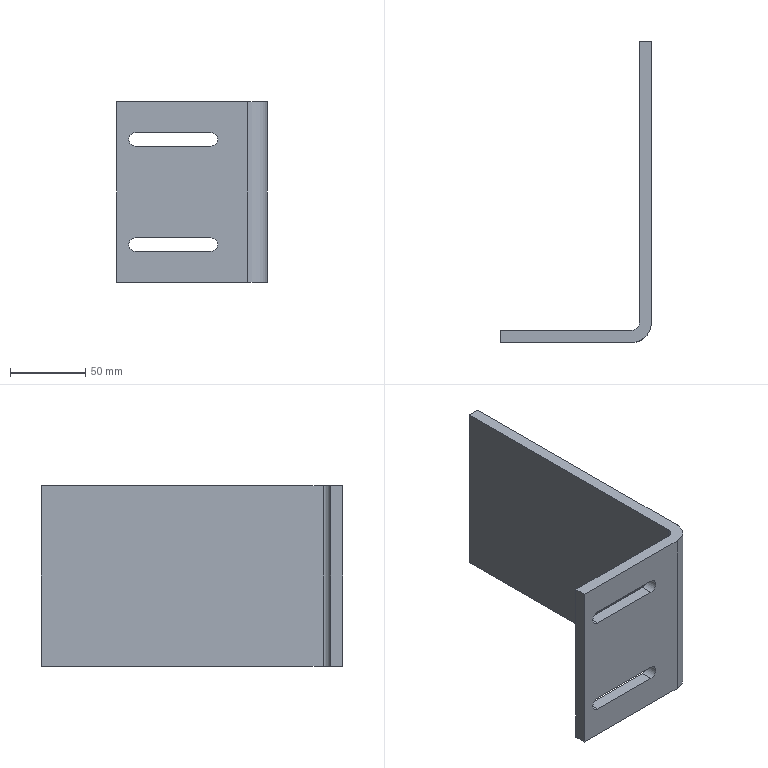Part | SolidWorks | features Extrusion 1, ICE 1 | 1 solid | 18 faces | box 100 x 200 x 120 mm | volume 268394 mm3 | plane 12 | cylinder 6 | commonest cylinder face diameters 9 x4 10 x1 26 x1
STEP:
#1=CARTESIAN_POINT('',(12.5,8.,20.5));
#2=VERTEX_POINT('',#1);
#3=CARTESIAN_POINT('',(12.5,8.,29.5));
#4=VERTEX_POINT('',#3);
#5=CARTESIAN_POINT('',(12.5,8.,25.));
#6=DIRECTION('',(0.,1.,0.));
#7=DIRECTION('',(0.,0.,1.));
#8=AXIS2_PLACEMENT_3D('',#5,#6,#7);
#9=CIRCLE('',#8,4.5);
#10=EDGE_CURVE('',#2,#4,#9,.T.);
#11=ORIENTED_EDGE('',*,*,#10,.F.);
#12=CARTESIAN_POINT('',(62.5,8.,20.5));
#13=VERTEX_POINT('',#12);
#14=CARTESIAN_POINT('',(12.5,8.,20.5));
#15=DIRECTION('',(-1.,0.,0.));
#16=VECTOR('',#15,1000.);
#17=LINE('',#14,#16);
#18=EDGE_CURVE('',#13,#2,#17,.T.);
#19=ORIENTED_EDGE('',*,*,#18,.F.);
#20=CARTESIAN_POINT('',(62.5,8.,29.5));
#21=VERTEX_POINT('',#20);
#22=CARTESIAN_POINT('',(62.5,8.,25.));
#23=DIRECTION('',(0.,1.,0.));
#24=DIRECTION('',(0.,0.,1.));
#25=AXIS2_PLACEMENT_3D('',#22,#23,#24);
#26=CIRCLE('',#25,4.5);
#27=EDGE_CURVE('',#21,#13,#26,.T.);
#28=ORIENTED_EDGE('',*,*,#27,.F.);
#29=CARTESIAN_POINT('',(12.5,8.,29.5));
#30=DIRECTION('',(1.,0.,0.));
#31=VECTOR('',#30,1000.);
#32=LINE('',#29,#31);
#33=EDGE_CURVE('',#4,#21,#32,.T.);
#34=ORIENTED_EDGE('',*,*,#33,.F.);
#35=EDGE_LOOP('',(#11,#19,#28,#34));
#36=FACE_BOUND('',#35,.T.);
#37=CARTESIAN_POINT('',(12.5,8.,90.5));
#38=VERTEX_POINT('',#37);
#39=CARTESIAN_POINT('',(12.5,8.,99.5));
#40=VERTEX_POINT('',#39);
#41=CARTESIAN_POINT('',(12.5,8.,95.));
#42=DIRECTION('',(0.,1.,0.));
#43=DIRECTION('',(0.,0.,-1.));
#44=AXIS2_PLACEMENT_3D('',#41,#42,#43);
#45=CIRCLE('',#44,4.5);
#46=EDGE_CURVE('',#38,#40,#45,.T.);
#47=ORIENTED_EDGE('',*,*,#46,.F.);
#48=CARTESIAN_POINT('',(62.5,8.,90.5));
#49=VERTEX_POINT('',#48);
#50=CARTESIAN_POINT('',(12.5,8.,90.5));
#51=DIRECTION('',(-1.,0.,0.));
#52=VECTOR('',#51,1000.);
#53=LINE('',#50,#52);
#54=EDGE_CURVE('',#49,#38,#53,.T.);
#55=ORIENTED_EDGE('',*,*,#54,.F.);
#56=CARTESIAN_POINT('',(62.5,8.,99.5));
#57=VERTEX_POINT('',#56);
#58=CARTESIAN_POINT('',(62.5,8.,95.));
#59=DIRECTION('',(0.,1.,0.));
#60=DIRECTION('',(0.,0.,-1.));
#61=AXIS2_PLACEMENT_3D('',#58,#59,#60);
#62=CIRCLE('',#61,4.5);
#63=EDGE_CURVE('',#57,#49,#62,.T.);
#64=ORIENTED_EDGE('',*,*,#63,.F.);
#65=CARTESIAN_POINT('',(12.5,8.,99.5));
#66=DIRECTION('',(1.,0.,0.));
#67=VECTOR('',#66,1000.);
#68=LINE('',#65,#67);
#69=EDGE_CURVE('',#40,#57,#68,.T.);
#70=ORIENTED_EDGE('',*,*,#69,.F.);
#71=EDGE_LOOP('',(#47,#55,#64,#70));
#72=FACE_BOUND('',#71,.T.);
#73=CARTESIAN_POINT('',(0.,8.,0.));
#74=VERTEX_POINT('',#73);
#75=CARTESIAN_POINT('',(87.,8.,0.));
#76=VERTEX_POINT('',#75);
#77=CARTESIAN_POINT('',(0.,8.,0.));
#78=DIRECTION('',(1.,0.,0.));
#79=VECTOR('',#78,1000.);
#80=LINE('',#77,#79);
#81=EDGE_CURVE('',#74,#76,#80,.T.);
#82=ORIENTED_EDGE('',*,*,#81,.F.);
#83=CARTESIAN_POINT('',(0.,8.,120.));
#84=VERTEX_POINT('',#83);
#85=CARTESIAN_POINT('',(0.,8.,120.));
#86=DIRECTION('',(0.,0.,-1.));
#87=VECTOR('',#86,1000.);
#88=LINE('',#85,#87);
#89=EDGE_CURVE('',#84,#74,#88,.T.);
#90=ORIENTED_EDGE('',*,*,#89,.F.);
#91=CARTESIAN_POINT('',(87.,8.,120.));
#92=VERTEX_POINT('',#91);
#93=CARTESIAN_POINT('',(0.,8.,120.));
#94=DIRECTION('',(1.,0.,0.));
#95=VECTOR('',#94,1000.);
#96=LINE('',#93,#95);
#97=EDGE_CURVE('',#84,#92,#96,.T.);
#98=ORIENTED_EDGE('',*,*,#97,.T.);
#99=CARTESIAN_POINT('',(87.,8.,120.));
#100=DIRECTION('',(0.,0.,-1.));
#101=VECTOR('',#100,1000.);
#102=LINE('',#99,#101);
#103=EDGE_CURVE('',#92,#76,#102,.T.);
#104=ORIENTED_EDGE('',*,*,#103,.T.);
#105=EDGE_LOOP('',(#82,#90,#98,#104));
#106=FACE_OUTER_BOUND('',#105,.T.);
#107=CARTESIAN_POINT('',(0.,8.,120.));
#108=DIRECTION('',(0.,1.,0.));
#109=DIRECTION('',(0.,0.,1.));
#110=AXIS2_PLACEMENT_3D('',#107,#108,#109);
#111=PLANE('',#110);
#112=ADVANCED_FACE('',(#36,#72,#106),#111,.T.);
#113=CARTESIAN_POINT('',(0.,0.,0.));
#114=VERTEX_POINT('',#113);
#115=CARTESIAN_POINT('',(0.,8.,0.));
#116=DIRECTION('',(0.,-1.,0.));
#117=VECTOR('',#116,1000.);
#118=LINE('',#115,#117);
#119=EDGE_CURVE('',#74,#114,#118,.T.);
#120=ORIENTED_EDGE('',*,*,#119,.T.);
#121=CARTESIAN_POINT('',(0.,0.,120.));
#122=VERTEX_POINT('',#121);
#123=CARTESIAN_POINT('',(0.,0.,120.));
#124=DIRECTION('',(0.,0.,-1.));
#125=VECTOR('',#124,1000.);
#126=LINE('',#123,#125);
#127=EDGE_CURVE('',#122,#114,#126,.T.);
#128=ORIENTED_EDGE('',*,*,#127,.F.);
#129=CARTESIAN_POINT('',(0.,8.,120.));
#130=DIRECTION('',(0.,-1.,0.));
#131=VECTOR('',#130,1000.);
#132=LINE('',#129,#131);
#133=EDGE_CURVE('',#84,#122,#132,.T.);
#134=ORIENTED_EDGE('',*,*,#133,.F.);
#135=ORIENTED_EDGE('',*,*,#89,.T.);
#136=EDGE_LOOP('',(#120,#128,#134,#135));
#137=FACE_OUTER_BOUND('',#136,.T.);
#138=CARTESIAN_POINT('',(0.,8.,120.));
#139=DIRECTION('',(1.,0.,0.));
#140=DIRECTION('',(0.,0.,-1.));
#141=AXIS2_PLACEMENT_3D('',#138,#139,#140);
#142=PLANE('',#141);
#143=ADVANCED_FACE('',(#137),#142,.F.);
#144=CARTESIAN_POINT('',(62.5,0.,20.5));
#145=VERTEX_POINT('',#144);
#146=CARTESIAN_POINT('',(12.5,0.,20.5));
#147=VERTEX_POINT('',#146);
#148=CARTESIAN_POINT('',(0.,0.,20.5));
#149=DIRECTION('',(-1.,0.,0.));
#150=VECTOR('',#149,1000.);
#151=LINE('',#148,#150);
#152=EDGE_CURVE('',#145,#147,#151,.T.);
#153=ORIENTED_EDGE('',*,*,#152,.T.);
#154=CARTESIAN_POINT('',(12.5,0.,29.5));
#155=VERTEX_POINT('',#154);
#156=CARTESIAN_POINT('',(12.5,0.,25.));
#157=DIRECTION('',(0.,1.,0.));
#158=DIRECTION('',(0.,0.,1.));
#159=AXIS2_PLACEMENT_3D('',#156,#157,#158);
#160=CIRCLE('',#159,4.5);
#161=EDGE_CURVE('',#147,#155,#160,.T.);
#162=ORIENTED_EDGE('',*,*,#161,.T.);
#163=CARTESIAN_POINT('',(62.5,0.,29.5));
#164=VERTEX_POINT('',#163);
#165=CARTESIAN_POINT('',(0.,0.,29.5));
#166=DIRECTION('',(1.,0.,0.));
#167=VECTOR('',#166,1000.);
#168=LINE('',#165,#167);
#169=EDGE_CURVE('',#155,#164,#168,.T.);
#170=ORIENTED_EDGE('',*,*,#169,.T.);
#171=CARTESIAN_POINT('',(62.5,0.,25.));
#172=DIRECTION('',(0.,1.,0.));
#173=DIRECTION('',(0.,0.,1.));
#174=AXIS2_PLACEMENT_3D('',#171,#172,#173);
#175=CIRCLE('',#174,4.5);
#176=EDGE_CURVE('',#164,#145,#175,.T.);
#177=ORIENTED_EDGE('',*,*,#176,.T.);
#178=EDGE_LOOP('',(#153,#162,#170,#177));
#179=FACE_BOUND('',#178,.T.);
#180=CARTESIAN_POINT('',(62.5,0.,90.5));
#181=VERTEX_POINT('',#180);
#182=CARTESIAN_POINT('',(12.5,0.,90.5));
#183=VERTEX_POINT('',#182);
#184=CARTESIAN_POINT('',(0.,0.,90.5));
#185=DIRECTION('',(-1.,0.,0.));
#186=VECTOR('',#185,1000.);
#187=LINE('',#184,#186);
#188=EDGE_CURVE('',#181,#183,#187,.T.);
#189=ORIENTED_EDGE('',*,*,#188,.T.);
#190=CARTESIAN_POINT('',(12.5,0.,99.5));
#191=VERTEX_POINT('',#190);
#192=CARTESIAN_POINT('',(12.5,0.,95.));
#193=DIRECTION('',(0.,1.,0.));
#194=DIRECTION('',(0.,0.,1.));
#195=AXIS2_PLACEMENT_3D('',#192,#193,#194);
#196=CIRCLE('',#195,4.5);
#197=EDGE_CURVE('',#183,#191,#196,.T.);
#198=ORIENTED_EDGE('',*,*,#197,.T.);
#199=CARTESIAN_POINT('',(62.5,0.,99.5));
#200=VERTEX_POINT('',#199);
#201=CARTESIAN_POINT('',(0.,0.,99.5));
#202=DIRECTION('',(1.,0.,0.));
#203=VECTOR('',#202,1000.);
#204=LINE('',#201,#203);
#205=EDGE_CURVE('',#191,#200,#204,.T.);
#206=ORIENTED_EDGE('',*,*,#205,.T.);
#207=CARTESIAN_POINT('',(62.5,0.,95.));
#208=DIRECTION('',(0.,1.,0.));
#209=DIRECTION('',(0.,0.,1.));
#210=AXIS2_PLACEMENT_3D('',#207,#208,#209);
#211=CIRCLE('',#210,4.5);
#212=EDGE_CURVE('',#200,#181,#211,.T.);
#213=ORIENTED_EDGE('',*,*,#212,.T.);
#214=EDGE_LOOP('',(#189,#198,#206,#213));
#215=FACE_BOUND('',#214,.T.);
#216=CARTESIAN_POINT('',(87.,0.,0.));
#217=VERTEX_POINT('',#216);
#218=CARTESIAN_POINT('',(0.,0.,0.));
#219=DIRECTION('',(1.,0.,0.));
#220=VECTOR('',#219,1000.);
#221=LINE('',#218,#220);
#222=EDGE_CURVE('',#114,#217,#221,.T.);
#223=ORIENTED_EDGE('',*,*,#222,.T.);
#224=CARTESIAN_POINT('',(87.,0.,120.));
#225=VERTEX_POINT('',#224);
#226=CARTESIAN_POINT('',(87.,0.,120.));
#227=DIRECTION('',(0.,0.,-1.));
#228=VECTOR('',#227,1000.);
#229=LINE('',#226,#228);
#230=EDGE_CURVE('',#225,#217,#229,.T.);
#231=ORIENTED_EDGE('',*,*,#230,.F.);
#232=CARTESIAN_POINT('',(0.,0.,120.));
#233=DIRECTION('',(1.,0.,0.));
#234=VECTOR('',#233,1000.);
#235=LINE('',#232,#234);
#236=EDGE_CURVE('',#122,#225,#235,.T.);
#237=ORIENTED_EDGE('',*,*,#236,.F.);
#238=ORIENTED_EDGE('',*,*,#127,.T.);
#239=EDGE_LOOP('',(#223,#231,#237,#238));
#240=FACE_OUTER_BOUND('',#239,.T.);
#241=CARTESIAN_POINT('',(0.,0.,120.));
#242=DIRECTION('',(0.,1.,0.));
#243=DIRECTION('',(0.,0.,1.));
#244=AXIS2_PLACEMENT_3D('',#241,#242,#243);
#245=PLANE('',#244);
#246=ADVANCED_FACE('',(#179,#215,#240),#245,.F.);
#247=CARTESIAN_POINT('',(100.,13.,0.));
#248=VERTEX_POINT('',#247);
#249=CARTESIAN_POINT('',(87.,13.,0.));
#250=DIRECTION('',(0.,0.,1.));
#251=DIRECTION('',(1.,0.,0.));
#252=AXIS2_PLACEMENT_3D('',#249,#250,#251);
#253=CIRCLE('',#252,13.);
#254=EDGE_CURVE('',#217,#248,#253,.T.);
#255=ORIENTED_EDGE('',*,*,#254,.T.);
#256=CARTESIAN_POINT('',(100.,13.,120.));
#257=VERTEX_POINT('',#256);
#258=CARTESIAN_POINT('',(100.,13.,120.));
#259=DIRECTION('',(0.,0.,-1.));
#260=VECTOR('',#259,1000.);
#261=LINE('',#258,#260);
#262=EDGE_CURVE('',#257,#248,#261,.T.);
#263=ORIENTED_EDGE('',*,*,#262,.F.);
#264=CARTESIAN_POINT('',(87.,13.,120.));
#265=DIRECTION('',(0.,0.,1.));
#266=DIRECTION('',(1.,0.,0.));
#267=AXIS2_PLACEMENT_3D('',#264,#265,#266);
#268=CIRCLE('',#267,13.);
#269=EDGE_CURVE('',#225,#257,#268,.T.);
#270=ORIENTED_EDGE('',*,*,#269,.F.);
#271=ORIENTED_EDGE('',*,*,#230,.T.);
#272=EDGE_LOOP('',(#255,#263,#270,#271));
#273=FACE_OUTER_BOUND('',#272,.T.);
#274=CARTESIAN_POINT('',(87.,13.,120.));
#275=DIRECTION('',(0.,0.,-1.));
#276=DIRECTION('',(-1.,0.,0.));
#277=AXIS2_PLACEMENT_3D('',#274,#275,#276);
#278=CYLINDRICAL_SURFACE('',#277,13.);
#279=ADVANCED_FACE('',(#273),#278,.T.);
#280=CARTESIAN_POINT('',(100.,200.,0.));
#281=VERTEX_POINT('',#280);
#282=CARTESIAN_POINT('',(100.,13.,0.));
#283=DIRECTION('',(0.,1.,0.));
#284=VECTOR('',#283,1000.);
#285=LINE('',#282,#284);
#286=EDGE_CURVE('',#248,#281,#285,.T.);
#287=ORIENTED_EDGE('',*,*,#286,.T.);
#288=CARTESIAN_POINT('',(100.,200.,120.));
#289=VERTEX_POINT('',#288);
#290=CARTESIAN_POINT('',(100.,200.,120.));
#291=DIRECTION('',(0.,0.,-1.));
#292=VECTOR('',#291,1000.);
#293=LINE('',#290,#292);
#294=EDGE_CURVE('',#289,#281,#293,.T.);
#295=ORIENTED_EDGE('',*,*,#294,.F.);
#296=CARTESIAN_POINT('',(100.,13.,120.));
#297=DIRECTION('',(0.,1.,0.));
#298=VECTOR('',#297,1000.);
#299=LINE('',#296,#298);
#300=EDGE_CURVE('',#257,#289,#299,.T.);
#301=ORIENTED_EDGE('',*,*,#300,.F.);
#302=ORIENTED_EDGE('',*,*,#262,.T.);
#303=EDGE_LOOP('',(#287,#295,#301,#302));
#304=FACE_OUTER_BOUND('',#303,.T.);
#305=CARTESIAN_POINT('',(100.,13.,120.));
#306=DIRECTION('',(-1.,0.,0.));
#307=DIRECTION('',(0.,0.,1.));
#308=AXIS2_PLACEMENT_3D('',#305,#306,#307);
#309=PLANE('',#308);
#310=ADVANCED_FACE('',(#304),#309,.F.);
#311=CARTESIAN_POINT('',(92.,200.,0.));
#312=VERTEX_POINT('',#311);
#313=CARTESIAN_POINT('',(100.,200.,0.));
#314=DIRECTION('',(-1.,0.,0.));
#315=VECTOR('',#314,1000.);
#316=LINE('',#313,#315);
#317=EDGE_CURVE('',#281,#312,#316,.T.);
#318=ORIENTED_EDGE('',*,*,#317,.T.);
#319=CARTESIAN_POINT('',(92.,200.,120.));
#320=VERTEX_POINT('',#319);
#321=CARTESIAN_POINT('',(92.,200.,120.));
#322=DIRECTION('',(0.,0.,-1.));
#323=VECTOR('',#322,1000.);
#324=LINE('',#321,#323);
#325=EDGE_CURVE('',#320,#312,#324,.T.);
#326=ORIENTED_EDGE('',*,*,#325,.F.);
#327=CARTESIAN_POINT('',(100.,200.,120.));
#328=DIRECTION('',(-1.,0.,0.));
#329=VECTOR('',#328,1000.);
#330=LINE('',#327,#329);
#331=EDGE_CURVE('',#289,#320,#330,.T.);
#332=ORIENTED_EDGE('',*,*,#331,.F.);
#333=ORIENTED_EDGE('',*,*,#294,.T.);
#334=EDGE_LOOP('',(#318,#326,#332,#333));
#335=FACE_OUTER_BOUND('',#334,.T.);
#336=CARTESIAN_POINT('',(100.,200.,120.));
#337=DIRECTION('',(0.,-1.,0.));
#338=DIRECTION('',(0.,0.,-1.));
#339=AXIS2_PLACEMENT_3D('',#336,#337,#338);
#340=PLANE('',#339);
#341=ADVANCED_FACE('',(#335),#340,.F.);
#342=CARTESIAN_POINT('',(92.,13.,0.));
#343=VERTEX_POINT('',#342);
#344=CARTESIAN_POINT('',(92.,13.,0.));
#345=DIRECTION('',(0.,1.,0.));
#346=VECTOR('',#345,1000.);
#347=LINE('',#344,#346);
#348=EDGE_CURVE('',#343,#312,#347,.T.);
#349=ORIENTED_EDGE('',*,*,#348,.F.);
#350=CARTESIAN_POINT('',(92.,13.,120.));
#351=VERTEX_POINT('',#350);
#352=CARTESIAN_POINT('',(92.,13.,120.));
#353=DIRECTION('',(0.,0.,-1.));
#354=VECTOR('',#353,1000.);
#355=LINE('',#352,#354);
#356=EDGE_CURVE('',#351,#343,#355,.T.);
#357=ORIENTED_EDGE('',*,*,#356,.F.);
#358=CARTESIAN_POINT('',(92.,13.,120.));
#359=DIRECTION('',(0.,1.,0.));
#360=VECTOR('',#359,1000.);
#361=LINE('',#358,#360);
#362=EDGE_CURVE('',#351,#320,#361,.T.);
#363=ORIENTED_EDGE('',*,*,#362,.T.);
#364=ORIENTED_EDGE('',*,*,#325,.T.);
#365=EDGE_LOOP('',(#349,#357,#363,#364));
#366=FACE_OUTER_BOUND('',#365,.T.);
#367=CARTESIAN_POINT('',(92.,13.,120.));
#368=DIRECTION('',(-1.,0.,0.));
#369=DIRECTION('',(0.,0.,1.));
#370=AXIS2_PLACEMENT_3D('',#367,#368,#369);
#371=PLANE('',#370);
#372=ADVANCED_FACE('',(#366),#371,.T.);
#373=CARTESIAN_POINT('',(87.,13.,0.));
#374=DIRECTION('',(0.,0.,1.));
#375=DIRECTION('',(1.,0.,0.));
#376=AXIS2_PLACEMENT_3D('',#373,#374,#375);
#377=CIRCLE('',#376,5.);
#378=EDGE_CURVE('',#76,#343,#377,.T.);
#379=ORIENTED_EDGE('',*,*,#378,.F.);
#380=ORIENTED_EDGE('',*,*,#103,.F.);
#381=CARTESIAN_POINT('',(87.,13.,120.));
#382=DIRECTION('',(0.,0.,1.));
#383=DIRECTION('',(1.,0.,0.));
#384=AXIS2_PLACEMENT_3D('',#381,#382,#383);
#385=CIRCLE('',#384,5.);
#386=EDGE_CURVE('',#92,#351,#385,.T.);
#387=ORIENTED_EDGE('',*,*,#386,.T.);
#388=ORIENTED_EDGE('',*,*,#356,.T.);
#389=EDGE_LOOP('',(#379,#380,#387,#388));
#390=FACE_OUTER_BOUND('',#389,.T.);
#391=CARTESIAN_POINT('',(87.,13.,120.));
#392=DIRECTION('',(0.,0.,-1.));
#393=DIRECTION('',(-1.,0.,0.));
#394=AXIS2_PLACEMENT_3D('',#391,#392,#393);
#395=CYLINDRICAL_SURFACE('',#394,5.);
#396=ADVANCED_FACE('',(#390),#395,.F.);
#397=ORIENTED_EDGE('',*,*,#97,.F.);
#398=ORIENTED_EDGE('',*,*,#133,.T.);
#399=ORIENTED_EDGE('',*,*,#236,.T.);
#400=ORIENTED_EDGE('',*,*,#269,.T.);
#401=ORIENTED_EDGE('',*,*,#300,.T.);
#402=ORIENTED_EDGE('',*,*,#331,.T.);
#403=ORIENTED_EDGE('',*,*,#362,.F.);
#404=ORIENTED_EDGE('',*,*,#386,.F.);
#405=EDGE_LOOP('',(#397,#398,#399,#400,#401,#402,#403,#404));
#406=FACE_OUTER_BOUND('',#405,.T.);
#407=CARTESIAN_POINT('',(87.,13.,120.));
#408=DIRECTION('',(0.,0.,1.));
#409=DIRECTION('',(1.,0.,0.));
#410=AXIS2_PLACEMENT_3D('',#407,#408,#409);
#411=PLANE('',#410);
#412=ADVANCED_FACE('',(#406),#411,.T.);
#413=ORIENTED_EDGE('',*,*,#81,.T.);
#414=ORIENTED_EDGE('',*,*,#378,.T.);
#415=ORIENTED_EDGE('',*,*,#348,.T.);
#416=ORIENTED_EDGE('',*,*,#317,.F.);
#417=ORIENTED_EDGE('',*,*,#286,.F.);
#418=ORIENTED_EDGE('',*,*,#254,.F.);
#419=ORIENTED_EDGE('',*,*,#222,.F.);
#420=ORIENTED_EDGE('',*,*,#119,.F.);
#421=EDGE_LOOP('',(#413,#414,#415,#416,#417,#418,#419,#420));
#422=FACE_OUTER_BOUND('',#421,.T.);
#423=CARTESIAN_POINT('',(87.,13.,0.));
#424=DIRECTION('',(0.,0.,1.));
#425=DIRECTION('',(1.,0.,0.));
#426=AXIS2_PLACEMENT_3D('',#423,#424,#425);
#427=PLANE('',#426);
#428=ADVANCED_FACE('',(#422),#427,.F.);
#429=CARTESIAN_POINT('',(12.5,-112.,90.5));
#430=DIRECTION('',(0.,1.,0.));
#431=VECTOR('',#430,1000.);
#432=LINE('',#429,#431);
#433=EDGE_CURVE('',#183,#38,#432,.T.);
#434=ORIENTED_EDGE('',*,*,#433,.T.);
#435=ORIENTED_EDGE('',*,*,#46,.T.);
#436=CARTESIAN_POINT('',(12.5,-112.,99.5));
#437=DIRECTION('',(0.,1.,0.));
#438=VECTOR('',#437,1000.);
#439=LINE('',#436,#438);
#440=EDGE_CURVE('',#191,#40,#439,.T.);
#441=ORIENTED_EDGE('',*,*,#440,.F.);
#442=ORIENTED_EDGE('',*,*,#197,.F.);
#443=EDGE_LOOP('',(#434,#435,#441,#442));
#444=FACE_OUTER_BOUND('',#443,.T.);
#445=CARTESIAN_POINT('',(12.5,-112.,95.));
#446=DIRECTION('',(0.,1.,0.));
#447=DIRECTION('',(0.,0.,1.));
#448=AXIS2_PLACEMENT_3D('',#445,#446,#447);
#449=CYLINDRICAL_SURFACE('',#448,4.5);
#450=ADVANCED_FACE('',(#444),#449,.F.);
#451=CARTESIAN_POINT('',(62.5,-112.,90.5));
#452=DIRECTION('',(0.,1.,0.));
#453=VECTOR('',#452,1000.);
#454=LINE('',#451,#453);
#455=EDGE_CURVE('',#181,#49,#454,.T.);
#456=ORIENTED_EDGE('',*,*,#455,.T.);
#457=ORIENTED_EDGE('',*,*,#54,.T.);
#458=ORIENTED_EDGE('',*,*,#433,.F.);
#459=ORIENTED_EDGE('',*,*,#188,.F.);
#460=EDGE_LOOP('',(#456,#457,#458,#459));
#461=FACE_OUTER_BOUND('',#460,.T.);
#462=CARTESIAN_POINT('',(12.5,-112.,90.5));
#463=DIRECTION('',(0.,0.,-1.));
#464=DIRECTION('',(-1.,0.,0.));
#465=AXIS2_PLACEMENT_3D('',#462,#463,#464);
#466=PLANE('',#465);
#467=ADVANCED_FACE('',(#461),#466,.F.);
#468=CARTESIAN_POINT('',(62.5,-112.,99.5));
#469=DIRECTION('',(0.,1.,0.));
#470=VECTOR('',#469,1000.);
#471=LINE('',#468,#470);
#472=EDGE_CURVE('',#200,#57,#471,.T.);
#473=ORIENTED_EDGE('',*,*,#472,.T.);
#474=ORIENTED_EDGE('',*,*,#63,.T.);
#475=ORIENTED_EDGE('',*,*,#455,.F.);
#476=ORIENTED_EDGE('',*,*,#212,.F.);
#477=EDGE_LOOP('',(#473,#474,#475,#476));
#478=FACE_OUTER_BOUND('',#477,.T.);
#479=CARTESIAN_POINT('',(62.5,-112.,95.));
#480=DIRECTION('',(0.,1.,0.));
#481=DIRECTION('',(0.,0.,1.));
#482=AXIS2_PLACEMENT_3D('',#479,#480,#481);
#483=CYLINDRICAL_SURFACE('',#482,4.5);
#484=ADVANCED_FACE('',(#478),#483,.F.);
#485=ORIENTED_EDGE('',*,*,#440,.T.);
#486=ORIENTED_EDGE('',*,*,#69,.T.);
#487=ORIENTED_EDGE('',*,*,#472,.F.);
#488=ORIENTED_EDGE('',*,*,#205,.F.);
#489=EDGE_LOOP('',(#485,#486,#487,#488));
#490=FACE_OUTER_BOUND('',#489,.T.);
#491=CARTESIAN_POINT('',(12.5,-112.,99.5));
#492=DIRECTION('',(0.,0.,1.));
#493=DIRECTION('',(1.,0.,0.));
#494=AXIS2_PLACEMENT_3D('',#491,#492,#493);
#495=PLANE('',#494);
#496=ADVANCED_FACE('',(#490),#495,.F.);
#497=CARTESIAN_POINT('',(12.5,-112.,20.5));
#498=DIRECTION('',(0.,1.,0.));
#499=VECTOR('',#498,1000.);
#500=LINE('',#497,#499);
#501=EDGE_CURVE('',#147,#2,#500,.T.);
#502=ORIENTED_EDGE('',*,*,#501,.T.);
#503=ORIENTED_EDGE('',*,*,#10,.T.);
#504=CARTESIAN_POINT('',(12.5,-112.,29.5));
#505=DIRECTION('',(0.,1.,0.));
#506=VECTOR('',#505,1000.);
#507=LINE('',#504,#506);
#508=EDGE_CURVE('',#155,#4,#507,.T.);
#509=ORIENTED_EDGE('',*,*,#508,.F.);
#510=ORIENTED_EDGE('',*,*,#161,.F.);
#511=EDGE_LOOP('',(#502,#503,#509,#510));
#512=FACE_OUTER_BOUND('',#511,.T.);
#513=CARTESIAN_POINT('',(12.5,-112.,25.));
#514=DIRECTION('',(0.,1.,0.));
#515=DIRECTION('',(0.,0.,1.));
#516=AXIS2_PLACEMENT_3D('',#513,#514,#515);
#517=CYLINDRICAL_SURFACE('',#516,4.5);
#518=ADVANCED_FACE('',(#512),#517,.F.);
#519=CARTESIAN_POINT('',(62.5,-112.,20.5));
#520=DIRECTION('',(0.,1.,0.));
#521=VECTOR('',#520,1000.);
#522=LINE('',#519,#521);
#523=EDGE_CURVE('',#145,#13,#522,.T.);
#524=ORIENTED_EDGE('',*,*,#523,.T.);
#525=ORIENTED_EDGE('',*,*,#18,.T.);
#526=ORIENTED_EDGE('',*,*,#501,.F.);
#527=ORIENTED_EDGE('',*,*,#152,.F.);
#528=EDGE_LOOP('',(#524,#525,#526,#527));
#529=FACE_OUTER_BOUND('',#528,.T.);
#530=CARTESIAN_POINT('',(12.5,-112.,20.5));
#531=DIRECTION('',(0.,0.,-1.));
#532=DIRECTION('',(-1.,0.,0.));
#533=AXIS2_PLACEMENT_3D('',#530,#531,#532);
#534=PLANE('',#533);
#535=ADVANCED_FACE('',(#529),#534,.F.);
#536=CARTESIAN_POINT('',(62.5,-112.,29.5));
#537=DIRECTION('',(0.,1.,0.));
#538=VECTOR('',#537,1000.);
#539=LINE('',#536,#538);
#540=EDGE_CURVE('',#164,#21,#539,.T.);
#541=ORIENTED_EDGE('',*,*,#540,.T.);
#542=ORIENTED_EDGE('',*,*,#27,.T.);
#543=ORIENTED_EDGE('',*,*,#523,.F.);
#544=ORIENTED_EDGE('',*,*,#176,.F.);
#545=EDGE_LOOP('',(#541,#542,#543,#544));
#546=FACE_OUTER_BOUND('',#545,.T.);
#547=CARTESIAN_POINT('',(62.5,-112.,25.));
#548=DIRECTION('',(0.,1.,0.));
#549=DIRECTION('',(0.,0.,1.));
#550=AXIS2_PLACEMENT_3D('',#547,#548,#549);
#551=CYLINDRICAL_SURFACE('',#550,4.5);
#552=ADVANCED_FACE('',(#546),#551,.F.);
#553=ORIENTED_EDGE('',*,*,#508,.T.);
#554=ORIENTED_EDGE('',*,*,#33,.T.);
#555=ORIENTED_EDGE('',*,*,#540,.F.);
#556=ORIENTED_EDGE('',*,*,#169,.F.);
#557=EDGE_LOOP('',(#553,#554,#555,#556));
#558=FACE_OUTER_BOUND('',#557,.T.);
#559=CARTESIAN_POINT('',(12.5,-112.,29.5));
#560=DIRECTION('',(0.,0.,1.));
#561=DIRECTION('',(1.,0.,0.));
#562=AXIS2_PLACEMENT_3D('',#559,#560,#561);
#563=PLANE('',#562);
#564=ADVANCED_FACE('',(#558),#563,.F.);
#565=CLOSED_SHELL('',(#112,#143,#246,#279,#310,#341,#372,#396,#412,#428,#450,#467,#484,#496,#518,#535,#552,#564));
#566=MANIFOLD_SOLID_BREP('',#565);
#567=CARTESIAN_POINT('',(0.,0.,0.));
#568=DIRECTION('',(0.,0.,1.));
#569=DIRECTION('',(1.,0.,0.));
#570=AXIS2_PLACEMENT_3D('',#567,#568,#569);
#571=(LENGTH_UNIT()NAMED_UNIT(*)SI_UNIT(.MILLI.,.METRE.));
#572=UNCERTAINTY_MEASURE_WITH_UNIT(LENGTH_MEASURE(0.00001),#571,'','');
#573=(NAMED_UNIT(*)PLANE_ANGLE_UNIT()SI_UNIT($,.RADIAN.));
#574=(NAMED_UNIT(*)SI_UNIT($,.STERADIAN.)SOLID_ANGLE_UNIT());
#575=(GEOMETRIC_REPRESENTATION_CONTEXT(3)GLOBAL_UNCERTAINTY_ASSIGNED_CONTEXT((#572))GLOBAL_UNIT_ASSIGNED_CONTEXT((#571,#573,#574))REPRESENTATION_CONTEXT('',''));
#576=ADVANCED_BREP_SHAPE_REPRESENTATION('',(#566,#570),#575);